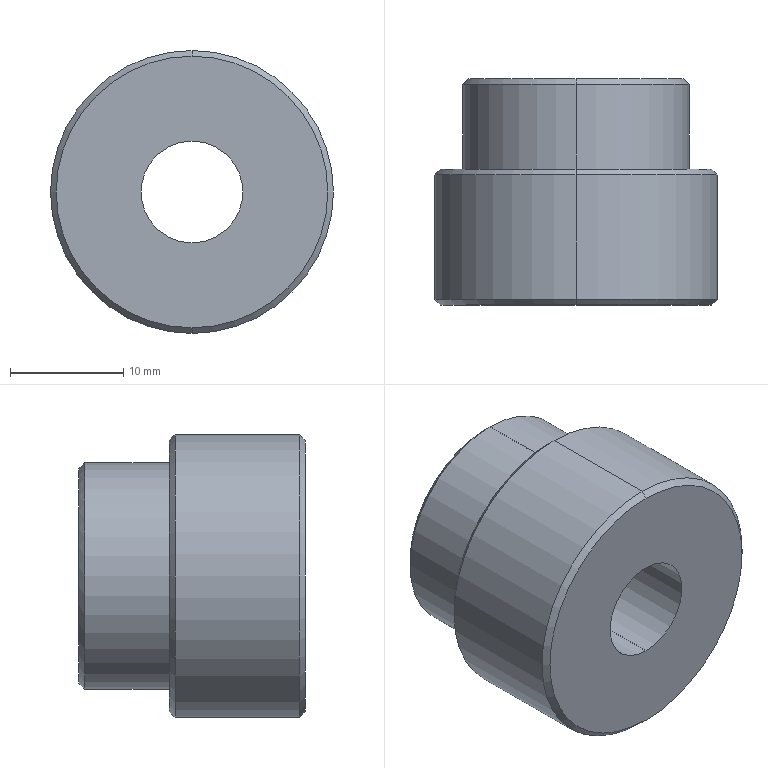Part | SolidWorks | features Chamfer 2, ICE 2, Extrusion 1 | 1 solid | 15 faces | box 25 x 20 x 25 mm | volume 7104 mm3 | cone 6 | cylinder 6 | plane 3 | commonest cylinder face diameters 9 x2 20 x2 25 x2
STEP:
#1=CARTESIAN_POINT('',(0.,20.,9.5));
#2=VERTEX_POINT('',#1);
#3=CARTESIAN_POINT('',(0.,20.,-9.5));
#4=VERTEX_POINT('',#3);
#5=CARTESIAN_POINT('',(0.,20.,0.));
#6=DIRECTION('',(0.,1.,0.));
#7=DIRECTION('',(0.,0.,1.));
#8=AXIS2_PLACEMENT_3D('',#5,#6,#7);
#9=CIRCLE('',#8,9.5);
#10=EDGE_CURVE('',#2,#4,#9,.T.);
#11=ORIENTED_EDGE('',*,*,#10,.F.);
#12=CARTESIAN_POINT('',(0.,19.5,10.));
#13=VERTEX_POINT('',#12);
#14=CARTESIAN_POINT('',(0.,20.,9.5));
#15=DIRECTION('',(0.,-0.7071,0.7071));
#16=VECTOR('',#15,1000.);
#17=LINE('',#14,#16);
#18=EDGE_CURVE('',#2,#13,#17,.T.);
#19=ORIENTED_EDGE('',*,*,#18,.T.);
#20=CARTESIAN_POINT('',(0.,19.5,-10.));
#21=VERTEX_POINT('',#20);
#22=CARTESIAN_POINT('',(0.,19.5,0.));
#23=DIRECTION('',(0.,-1.,0.));
#24=DIRECTION('',(0.,0.,1.));
#25=AXIS2_PLACEMENT_3D('',#22,#23,#24);
#26=CIRCLE('',#25,10.);
#27=EDGE_CURVE('',#21,#13,#26,.T.);
#28=ORIENTED_EDGE('',*,*,#27,.F.);
#29=CARTESIAN_POINT('',(0.,20.,-9.5));
#30=DIRECTION('',(0.,-0.7071,-0.7071));
#31=VECTOR('',#30,1000.);
#32=LINE('',#29,#31);
#33=EDGE_CURVE('',#4,#21,#32,.T.);
#34=ORIENTED_EDGE('',*,*,#33,.F.);
#35=EDGE_LOOP('',(#11,#19,#28,#34));
#36=FACE_OUTER_BOUND('',#35,.T.);
#37=CARTESIAN_POINT('',(0.,20.,0.));
#38=DIRECTION('',(0.,-1.,0.));
#39=DIRECTION('',(0.,0.,-1.));
#40=AXIS2_PLACEMENT_3D('',#37,#38,#39);
#41=CONICAL_SURFACE('',#40,9.5,0.7854);
#42=ADVANCED_FACE('',(#36),#41,.T.);
#43=CARTESIAN_POINT('',(0.,12.,12.));
#44=VERTEX_POINT('',#43);
#45=CARTESIAN_POINT('',(0.,12.,-12.));
#46=VERTEX_POINT('',#45);
#47=CARTESIAN_POINT('',(0.,12.,0.));
#48=DIRECTION('',(0.,1.,0.));
#49=DIRECTION('',(0.,0.,-1.));
#50=AXIS2_PLACEMENT_3D('',#47,#48,#49);
#51=CIRCLE('',#50,12.);
#52=EDGE_CURVE('',#44,#46,#51,.T.);
#53=ORIENTED_EDGE('',*,*,#52,.F.);
#54=CARTESIAN_POINT('',(0.,11.5,12.5));
#55=VERTEX_POINT('',#54);
#56=CARTESIAN_POINT('',(0.,11.5,12.5));
#57=DIRECTION('',(0.,-0.7071,0.7071));
#58=VECTOR('',#57,1000.);
#59=LINE('',#56,#58);
#60=EDGE_CURVE('',#44,#55,#59,.T.);
#61=ORIENTED_EDGE('',*,*,#60,.T.);
#62=CARTESIAN_POINT('',(0.,11.5,-12.5));
#63=VERTEX_POINT('',#62);
#64=CARTESIAN_POINT('',(0.,11.5,0.));
#65=DIRECTION('',(0.,-1.,0.));
#66=DIRECTION('',(0.,0.,-1.));
#67=AXIS2_PLACEMENT_3D('',#64,#65,#66);
#68=CIRCLE('',#67,12.5);
#69=EDGE_CURVE('',#63,#55,#68,.T.);
#70=ORIENTED_EDGE('',*,*,#69,.F.);
#71=CARTESIAN_POINT('',(0.,11.5,-12.5));
#72=DIRECTION('',(0.,-0.7071,-0.7071));
#73=VECTOR('',#72,1000.);
#74=LINE('',#71,#73);
#75=EDGE_CURVE('',#46,#63,#74,.T.);
#76=ORIENTED_EDGE('',*,*,#75,.F.);
#77=EDGE_LOOP('',(#53,#61,#70,#76));
#78=FACE_OUTER_BOUND('',#77,.T.);
#79=CARTESIAN_POINT('',(0.,11.5,0.));
#80=DIRECTION('',(0.,-1.,0.));
#81=DIRECTION('',(0.,0.,-1.));
#82=AXIS2_PLACEMENT_3D('',#79,#80,#81);
#83=CONICAL_SURFACE('',#82,12.5,0.7854);
#84=ADVANCED_FACE('',(#78),#83,.T.);
#85=CARTESIAN_POINT('',(0.,0.,-12.));
#86=VERTEX_POINT('',#85);
#87=CARTESIAN_POINT('',(0.,0.,12.));
#88=VERTEX_POINT('',#87);
#89=CARTESIAN_POINT('',(0.,0.,0.));
#90=DIRECTION('',(0.,-1.,0.));
#91=DIRECTION('',(0.,0.,1.));
#92=AXIS2_PLACEMENT_3D('',#89,#90,#91);
#93=CIRCLE('',#92,12.);
#94=EDGE_CURVE('',#86,#88,#93,.T.);
#95=ORIENTED_EDGE('',*,*,#94,.F.);
#96=CARTESIAN_POINT('',(0.,0.5,-12.5));
#97=VERTEX_POINT('',#96);
#98=CARTESIAN_POINT('',(0.,0.,-12.));
#99=DIRECTION('',(0.,0.7071,-0.7071));
#100=VECTOR('',#99,1000.);
#101=LINE('',#98,#100);
#102=EDGE_CURVE('',#86,#97,#101,.T.);
#103=ORIENTED_EDGE('',*,*,#102,.T.);
#104=CARTESIAN_POINT('',(0.,0.5,12.5));
#105=VERTEX_POINT('',#104);
#106=CARTESIAN_POINT('',(0.,0.5,0.));
#107=DIRECTION('',(0.,1.,0.));
#108=DIRECTION('',(0.,0.,1.));
#109=AXIS2_PLACEMENT_3D('',#106,#107,#108);
#110=CIRCLE('',#109,12.5);
#111=EDGE_CURVE('',#105,#97,#110,.T.);
#112=ORIENTED_EDGE('',*,*,#111,.F.);
#113=CARTESIAN_POINT('',(0.,0.,12.));
#114=DIRECTION('',(0.,0.7071,0.7071));
#115=VECTOR('',#114,1000.);
#116=LINE('',#113,#115);
#117=EDGE_CURVE('',#88,#105,#116,.T.);
#118=ORIENTED_EDGE('',*,*,#117,.F.);
#119=EDGE_LOOP('',(#95,#103,#112,#118));
#120=FACE_OUTER_BOUND('',#119,.T.);
#121=CARTESIAN_POINT('',(0.,0.,0.));
#122=DIRECTION('',(0.,1.,0.));
#123=DIRECTION('',(0.,0.,1.));
#124=AXIS2_PLACEMENT_3D('',#121,#122,#123);
#125=CONICAL_SURFACE('',#124,12.,0.7854);
#126=ADVANCED_FACE('',(#120),#125,.T.);
#127=CARTESIAN_POINT('',(0.,0.,-4.5));
#128=VERTEX_POINT('',#127);
#129=CARTESIAN_POINT('',(0.,0.,4.5));
#130=VERTEX_POINT('',#129);
#131=CARTESIAN_POINT('',(0.,0.,0.));
#132=DIRECTION('',(0.,1.,0.));
#133=DIRECTION('',(0.,0.,1.));
#134=AXIS2_PLACEMENT_3D('',#131,#132,#133);
#135=CIRCLE('',#134,4.5);
#136=EDGE_CURVE('',#128,#130,#135,.T.);
#137=ORIENTED_EDGE('',*,*,#136,.F.);
#138=CARTESIAN_POINT('',(0.,20.,-4.5));
#139=VERTEX_POINT('',#138);
#140=CARTESIAN_POINT('',(0.,0.,-4.5));
#141=DIRECTION('',(0.,1.,0.));
#142=VECTOR('',#141,1000.);
#143=LINE('',#140,#142);
#144=EDGE_CURVE('',#128,#139,#143,.T.);
#145=ORIENTED_EDGE('',*,*,#144,.T.);
#146=CARTESIAN_POINT('',(0.,20.,4.5));
#147=VERTEX_POINT('',#146);
#148=CARTESIAN_POINT('',(0.,20.,0.));
#149=DIRECTION('',(0.,1.,0.));
#150=DIRECTION('',(0.,0.,1.));
#151=AXIS2_PLACEMENT_3D('',#148,#149,#150);
#152=CIRCLE('',#151,4.5);
#153=EDGE_CURVE('',#139,#147,#152,.T.);
#154=ORIENTED_EDGE('',*,*,#153,.T.);
#155=CARTESIAN_POINT('',(0.,0.,4.5));
#156=DIRECTION('',(0.,1.,0.));
#157=VECTOR('',#156,1000.);
#158=LINE('',#155,#157);
#159=EDGE_CURVE('',#130,#147,#158,.T.);
#160=ORIENTED_EDGE('',*,*,#159,.F.);
#161=EDGE_LOOP('',(#137,#145,#154,#160));
#162=FACE_OUTER_BOUND('',#161,.T.);
#163=CARTESIAN_POINT('',(0.,0.,0.));
#164=DIRECTION('',(0.,1.,0.));
#165=DIRECTION('',(0.,0.,1.));
#166=AXIS2_PLACEMENT_3D('',#163,#164,#165);
#167=CYLINDRICAL_SURFACE('',#166,4.5);
#168=ADVANCED_FACE('',(#162),#167,.F.);
#169=ORIENTED_EDGE('',*,*,#69,.T.);
#170=CARTESIAN_POINT('',(0.,12.,12.5));
#171=DIRECTION('',(0.,-1.,0.));
#172=VECTOR('',#171,1000.);
#173=LINE('',#170,#172);
#174=EDGE_CURVE('',#55,#105,#173,.T.);
#175=ORIENTED_EDGE('',*,*,#174,.T.);
#176=ORIENTED_EDGE('',*,*,#111,.T.);
#177=CARTESIAN_POINT('',(0.,12.,-12.5));
#178=DIRECTION('',(0.,-1.,0.));
#179=VECTOR('',#178,1000.);
#180=LINE('',#177,#179);
#181=EDGE_CURVE('',#63,#97,#180,.T.);
#182=ORIENTED_EDGE('',*,*,#181,.F.);
#183=EDGE_LOOP('',(#169,#175,#176,#182));
#184=FACE_OUTER_BOUND('',#183,.T.);
#185=CARTESIAN_POINT('',(0.,12.,0.));
#186=DIRECTION('',(0.,-1.,0.));
#187=DIRECTION('',(0.,0.,-1.));
#188=AXIS2_PLACEMENT_3D('',#185,#186,#187);
#189=CYLINDRICAL_SURFACE('',#188,12.5);
#190=ADVANCED_FACE('',(#184),#189,.T.);
#191=ORIENTED_EDGE('',*,*,#27,.T.);
#192=CARTESIAN_POINT('',(0.,12.,10.));
#193=VERTEX_POINT('',#192);
#194=CARTESIAN_POINT('',(0.,20.,10.));
#195=DIRECTION('',(0.,-1.,0.));
#196=VECTOR('',#195,1000.);
#197=LINE('',#194,#196);
#198=EDGE_CURVE('',#13,#193,#197,.T.);
#199=ORIENTED_EDGE('',*,*,#198,.T.);
#200=CARTESIAN_POINT('',(0.,12.,-10.));
#201=VERTEX_POINT('',#200);
#202=CARTESIAN_POINT('',(0.,12.,0.));
#203=DIRECTION('',(0.,-1.,0.));
#204=DIRECTION('',(0.,0.,-1.));
#205=AXIS2_PLACEMENT_3D('',#202,#203,#204);
#206=CIRCLE('',#205,10.);
#207=EDGE_CURVE('',#201,#193,#206,.T.);
#208=ORIENTED_EDGE('',*,*,#207,.F.);
#209=CARTESIAN_POINT('',(0.,20.,-10.));
#210=DIRECTION('',(0.,-1.,0.));
#211=VECTOR('',#210,1000.);
#212=LINE('',#209,#211);
#213=EDGE_CURVE('',#21,#201,#212,.T.);
#214=ORIENTED_EDGE('',*,*,#213,.F.);
#215=EDGE_LOOP('',(#191,#199,#208,#214));
#216=FACE_OUTER_BOUND('',#215,.T.);
#217=CARTESIAN_POINT('',(0.,20.,0.));
#218=DIRECTION('',(0.,-1.,0.));
#219=DIRECTION('',(0.,0.,-1.));
#220=AXIS2_PLACEMENT_3D('',#217,#218,#219);
#221=CYLINDRICAL_SURFACE('',#220,10.);
#222=ADVANCED_FACE('',(#216),#221,.T.);
#223=ORIENTED_EDGE('',*,*,#198,.F.);
#224=CARTESIAN_POINT('',(0.,19.5,0.));
#225=DIRECTION('',(0.,-1.,0.));
#226=DIRECTION('',(0.,0.,1.));
#227=AXIS2_PLACEMENT_3D('',#224,#225,#226);
#228=CIRCLE('',#227,10.);
#229=EDGE_CURVE('',#13,#21,#228,.T.);
#230=ORIENTED_EDGE('',*,*,#229,.T.);
#231=ORIENTED_EDGE('',*,*,#213,.T.);
#232=CARTESIAN_POINT('',(0.,12.,0.));
#233=DIRECTION('',(0.,-1.,0.));
#234=DIRECTION('',(0.,0.,-1.));
#235=AXIS2_PLACEMENT_3D('',#232,#233,#234);
#236=CIRCLE('',#235,10.);
#237=EDGE_CURVE('',#193,#201,#236,.T.);
#238=ORIENTED_EDGE('',*,*,#237,.F.);
#239=EDGE_LOOP('',(#223,#230,#231,#238));
#240=FACE_OUTER_BOUND('',#239,.T.);
#241=CARTESIAN_POINT('',(0.,20.,0.));
#242=DIRECTION('',(0.,-1.,0.));
#243=DIRECTION('',(0.,0.,-1.));
#244=AXIS2_PLACEMENT_3D('',#241,#242,#243);
#245=CYLINDRICAL_SURFACE('',#244,10.);
#246=ADVANCED_FACE('',(#240),#245,.T.);
#247=CARTESIAN_POINT('',(0.,20.,0.));
#248=DIRECTION('',(0.,1.,0.));
#249=DIRECTION('',(0.,0.,1.));
#250=AXIS2_PLACEMENT_3D('',#247,#248,#249);
#251=CIRCLE('',#250,9.5);
#252=EDGE_CURVE('',#4,#2,#251,.T.);
#253=ORIENTED_EDGE('',*,*,#252,.T.);
#254=ORIENTED_EDGE('',*,*,#10,.T.);
#255=EDGE_LOOP('',(#253,#254));
#256=FACE_OUTER_BOUND('',#255,.T.);
#257=CARTESIAN_POINT('',(0.,20.,0.));
#258=DIRECTION('',(0.,1.,0.));
#259=DIRECTION('',(0.,0.,1.));
#260=AXIS2_PLACEMENT_3D('',#257,#258,#259);
#261=CIRCLE('',#260,4.5);
#262=EDGE_CURVE('',#147,#139,#261,.T.);
#263=ORIENTED_EDGE('',*,*,#262,.F.);
#264=ORIENTED_EDGE('',*,*,#153,.F.);
#265=EDGE_LOOP('',(#263,#264));
#266=FACE_BOUND('',#265,.T.);
#267=CARTESIAN_POINT('',(0.,20.,0.));
#268=DIRECTION('',(0.,1.,0.));
#269=DIRECTION('',(0.,0.,1.));
#270=AXIS2_PLACEMENT_3D('',#267,#268,#269);
#271=PLANE('',#270);
#272=ADVANCED_FACE('',(#256,#266),#271,.T.);
#273=ORIENTED_EDGE('',*,*,#174,.F.);
#274=CARTESIAN_POINT('',(0.,11.5,0.));
#275=DIRECTION('',(0.,-1.,0.));
#276=DIRECTION('',(0.,0.,-1.));
#277=AXIS2_PLACEMENT_3D('',#274,#275,#276);
#278=CIRCLE('',#277,12.5);
#279=EDGE_CURVE('',#55,#63,#278,.T.);
#280=ORIENTED_EDGE('',*,*,#279,.T.);
#281=ORIENTED_EDGE('',*,*,#181,.T.);
#282=CARTESIAN_POINT('',(0.,0.5,0.));
#283=DIRECTION('',(0.,1.,0.));
#284=DIRECTION('',(0.,0.,1.));
#285=AXIS2_PLACEMENT_3D('',#282,#283,#284);
#286=CIRCLE('',#285,12.5);
#287=EDGE_CURVE('',#97,#105,#286,.T.);
#288=ORIENTED_EDGE('',*,*,#287,.T.);
#289=EDGE_LOOP('',(#273,#280,#281,#288));
#290=FACE_OUTER_BOUND('',#289,.T.);
#291=CARTESIAN_POINT('',(0.,12.,0.));
#292=DIRECTION('',(0.,-1.,0.));
#293=DIRECTION('',(0.,0.,-1.));
#294=AXIS2_PLACEMENT_3D('',#291,#292,#293);
#295=CYLINDRICAL_SURFACE('',#294,12.5);
#296=ADVANCED_FACE('',(#290),#295,.T.);
#297=CARTESIAN_POINT('',(0.,12.,0.));
#298=DIRECTION('',(0.,1.,0.));
#299=DIRECTION('',(0.,0.,-1.));
#300=AXIS2_PLACEMENT_3D('',#297,#298,#299);
#301=CIRCLE('',#300,12.);
#302=EDGE_CURVE('',#46,#44,#301,.T.);
#303=ORIENTED_EDGE('',*,*,#302,.T.);
#304=ORIENTED_EDGE('',*,*,#52,.T.);
#305=EDGE_LOOP('',(#303,#304));
#306=FACE_OUTER_BOUND('',#305,.T.);
#307=ORIENTED_EDGE('',*,*,#207,.T.);
#308=ORIENTED_EDGE('',*,*,#237,.T.);
#309=EDGE_LOOP('',(#307,#308));
#310=FACE_BOUND('',#309,.T.);
#311=CARTESIAN_POINT('',(0.,12.,0.));
#312=DIRECTION('',(0.,-1.,0.));
#313=DIRECTION('',(0.,0.,-1.));
#314=AXIS2_PLACEMENT_3D('',#311,#312,#313);
#315=PLANE('',#314);
#316=ADVANCED_FACE('',(#306,#310),#315,.F.);
#317=CARTESIAN_POINT('',(0.,0.,0.));
#318=DIRECTION('',(0.,-1.,0.));
#319=DIRECTION('',(0.,0.,1.));
#320=AXIS2_PLACEMENT_3D('',#317,#318,#319);
#321=CIRCLE('',#320,12.);
#322=EDGE_CURVE('',#88,#86,#321,.T.);
#323=ORIENTED_EDGE('',*,*,#322,.T.);
#324=ORIENTED_EDGE('',*,*,#94,.T.);
#325=EDGE_LOOP('',(#323,#324));
#326=FACE_OUTER_BOUND('',#325,.T.);
#327=CARTESIAN_POINT('',(0.,0.,0.));
#328=DIRECTION('',(0.,1.,0.));
#329=DIRECTION('',(0.,0.,1.));
#330=AXIS2_PLACEMENT_3D('',#327,#328,#329);
#331=CIRCLE('',#330,4.5);
#332=EDGE_CURVE('',#130,#128,#331,.T.);
#333=ORIENTED_EDGE('',*,*,#332,.T.);
#334=ORIENTED_EDGE('',*,*,#136,.T.);
#335=EDGE_LOOP('',(#333,#334));
#336=FACE_BOUND('',#335,.T.);
#337=CARTESIAN_POINT('',(0.,0.,0.));
#338=DIRECTION('',(0.,1.,0.));
#339=DIRECTION('',(0.,0.,1.));
#340=AXIS2_PLACEMENT_3D('',#337,#338,#339);
#341=PLANE('',#340);
#342=ADVANCED_FACE('',(#326,#336),#341,.F.);
#343=ORIENTED_EDGE('',*,*,#144,.F.);
#344=ORIENTED_EDGE('',*,*,#332,.F.);
#345=ORIENTED_EDGE('',*,*,#159,.T.);
#346=ORIENTED_EDGE('',*,*,#262,.T.);
#347=EDGE_LOOP('',(#343,#344,#345,#346));
#348=FACE_OUTER_BOUND('',#347,.T.);
#349=CARTESIAN_POINT('',(0.,0.,0.));
#350=DIRECTION('',(0.,1.,0.));
#351=DIRECTION('',(0.,0.,1.));
#352=AXIS2_PLACEMENT_3D('',#349,#350,#351);
#353=CYLINDRICAL_SURFACE('',#352,4.5);
#354=ADVANCED_FACE('',(#348),#353,.F.);
#355=ORIENTED_EDGE('',*,*,#102,.F.);
#356=ORIENTED_EDGE('',*,*,#322,.F.);
#357=ORIENTED_EDGE('',*,*,#117,.T.);
#358=ORIENTED_EDGE('',*,*,#287,.F.);
#359=EDGE_LOOP('',(#355,#356,#357,#358));
#360=FACE_OUTER_BOUND('',#359,.T.);
#361=CARTESIAN_POINT('',(0.,0.,0.));
#362=DIRECTION('',(0.,1.,0.));
#363=DIRECTION('',(0.,0.,1.));
#364=AXIS2_PLACEMENT_3D('',#361,#362,#363);
#365=CONICAL_SURFACE('',#364,12.,0.7854);
#366=ADVANCED_FACE('',(#360),#365,.T.);
#367=ORIENTED_EDGE('',*,*,#60,.F.);
#368=ORIENTED_EDGE('',*,*,#302,.F.);
#369=ORIENTED_EDGE('',*,*,#75,.T.);
#370=ORIENTED_EDGE('',*,*,#279,.F.);
#371=EDGE_LOOP('',(#367,#368,#369,#370));
#372=FACE_OUTER_BOUND('',#371,.T.);
#373=CARTESIAN_POINT('',(0.,11.5,0.));
#374=DIRECTION('',(0.,-1.,0.));
#375=DIRECTION('',(0.,0.,-1.));
#376=AXIS2_PLACEMENT_3D('',#373,#374,#375);
#377=CONICAL_SURFACE('',#376,12.5,0.7854);
#378=ADVANCED_FACE('',(#372),#377,.T.);
#379=ORIENTED_EDGE('',*,*,#18,.F.);
#380=ORIENTED_EDGE('',*,*,#252,.F.);
#381=ORIENTED_EDGE('',*,*,#33,.T.);
#382=ORIENTED_EDGE('',*,*,#229,.F.);
#383=EDGE_LOOP('',(#379,#380,#381,#382));
#384=FACE_OUTER_BOUND('',#383,.T.);
#385=CARTESIAN_POINT('',(0.,20.,0.));
#386=DIRECTION('',(0.,-1.,0.));
#387=DIRECTION('',(0.,0.,-1.));
#388=AXIS2_PLACEMENT_3D('',#385,#386,#387);
#389=CONICAL_SURFACE('',#388,9.5,0.7854);
#390=ADVANCED_FACE('',(#384),#389,.T.);
#391=CLOSED_SHELL('',(#42,#84,#126,#168,#190,#222,#246,#272,#296,#316,#342,#354,#366,#378,#390));
#392=MANIFOLD_SOLID_BREP('',#391);
#393=CARTESIAN_POINT('',(0.,0.,0.));
#394=DIRECTION('',(0.,0.,1.));
#395=DIRECTION('',(1.,0.,0.));
#396=AXIS2_PLACEMENT_3D('',#393,#394,#395);
#397=(LENGTH_UNIT()NAMED_UNIT(*)SI_UNIT(.MILLI.,.METRE.));
#398=UNCERTAINTY_MEASURE_WITH_UNIT(LENGTH_MEASURE(0.00001),#397,'','');
#399=(NAMED_UNIT(*)PLANE_ANGLE_UNIT()SI_UNIT($,.RADIAN.));
#400=(NAMED_UNIT(*)SI_UNIT($,.STERADIAN.)SOLID_ANGLE_UNIT());
#401=(GEOMETRIC_REPRESENTATION_CONTEXT(3)GLOBAL_UNCERTAINTY_ASSIGNED_CONTEXT((#398))GLOBAL_UNIT_ASSIGNED_CONTEXT((#397,#399,#400))REPRESENTATION_CONTEXT('',''));
#402=ADVANCED_BREP_SHAPE_REPRESENTATION('',(#392,#396),#401);